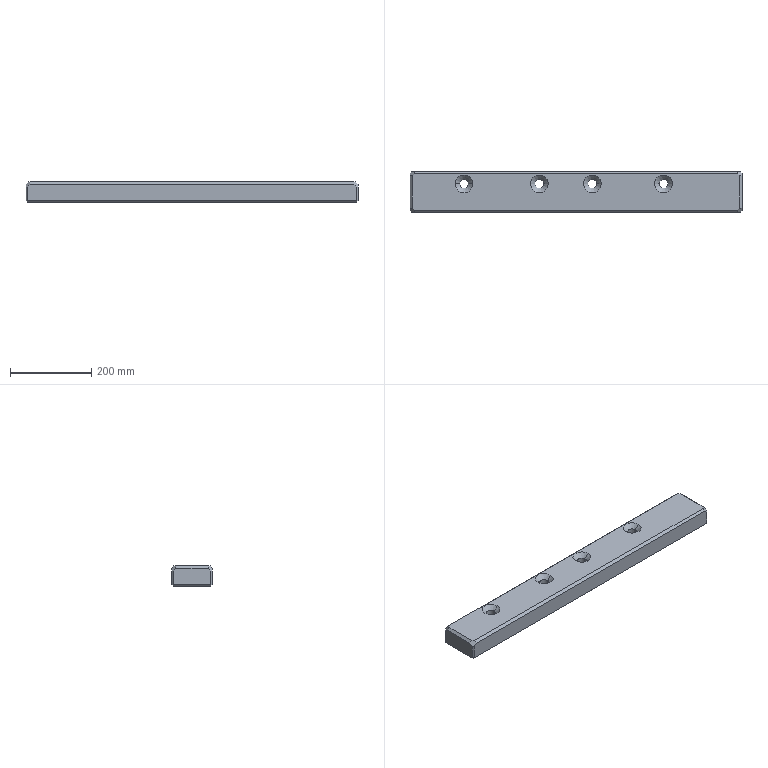Part | Creo | 1 solid | 50 faces | box 815 x 100 x 49.3 mm | volume 3878023 mm3 | plane 26 | cone 16 | cylinder 8 | commonest cylinder face diameters 22 x8
STEP:
#1=CARTESIAN_POINT('',(0.,0.,0.));
#2=DIRECTION('',(0.,0.,1.));
#3=DIRECTION('',(1.,0.,0.));
#4=AXIS2_PLACEMENT_3D('',#1,#2,#3);
#5=CARTESIAN_POINT('',(-330.17,-424.056,305.059));
#6=VERTEX_POINT('',#5);
#7=CARTESIAN_POINT('',(-325.328,-428.899,305.059));
#8=VERTEX_POINT('',#7);
#9=CARTESIAN_POINT('',(-330.17,-424.056,305.059));
#10=DIRECTION('',(0.7071,-0.7071,0.));
#11=VECTOR('',#10,6.848);
#12=LINE('',#9,#11);
#13=EDGE_CURVE('',#6,#8,#12,.T.);
#14=ORIENTED_EDGE('',*,*,#13,.F.);
#15=CARTESIAN_POINT('',(-330.17,-345.199,305.059));
#16=VERTEX_POINT('',#15);
#17=CARTESIAN_POINT('',(-330.17,-424.056,305.059));
#18=DIRECTION('',(0.,1.,0.));
#19=VECTOR('',#18,78.858);
#20=LINE('',#17,#19);
#21=EDGE_CURVE('',#6,#16,#20,.T.);
#22=ORIENTED_EDGE('',*,*,#21,.T.);
#23=CARTESIAN_POINT('',(-325.328,-340.356,305.059));
#24=VERTEX_POINT('',#23);
#25=CARTESIAN_POINT('',(-330.17,-345.199,305.059));
#26=DIRECTION('',(0.7071,0.7071,0.));
#27=VECTOR('',#26,6.848);
#28=LINE('',#25,#27);
#29=EDGE_CURVE('',#16,#24,#28,.T.);
#30=ORIENTED_EDGE('',*,*,#29,.T.);
#31=CARTESIAN_POINT('',(468.53,-340.356,305.059));
#32=VERTEX_POINT('',#31);
#33=CARTESIAN_POINT('',(-325.328,-340.356,305.059));
#34=DIRECTION('',(1.,0.,0.));
#35=VECTOR('',#34,793.858);
#36=LINE('',#33,#35);
#37=EDGE_CURVE('',#24,#32,#36,.T.);
#38=ORIENTED_EDGE('',*,*,#37,.T.);
#39=CARTESIAN_POINT('',(473.372,-345.199,305.059));
#40=VERTEX_POINT('',#39);
#41=CARTESIAN_POINT('',(473.372,-345.199,305.059));
#42=DIRECTION('',(-0.7071,0.7071,0.));
#43=VECTOR('',#42,6.848);
#44=LINE('',#41,#43);
#45=EDGE_CURVE('',#40,#32,#44,.T.);
#46=ORIENTED_EDGE('',*,*,#45,.F.);
#47=CARTESIAN_POINT('',(473.372,-424.056,305.059));
#48=VERTEX_POINT('',#47);
#49=CARTESIAN_POINT('',(473.372,-345.199,305.059));
#50=DIRECTION('',(0.,-1.,0.));
#51=VECTOR('',#50,78.858);
#52=LINE('',#49,#51);
#53=EDGE_CURVE('',#40,#48,#52,.T.);
#54=ORIENTED_EDGE('',*,*,#53,.T.);
#55=CARTESIAN_POINT('',(468.53,-428.899,305.059));
#56=VERTEX_POINT('',#55);
#57=CARTESIAN_POINT('',(468.53,-428.899,305.059));
#58=DIRECTION('',(0.7071,0.7071,0.));
#59=VECTOR('',#58,6.848);
#60=LINE('',#57,#59);
#61=EDGE_CURVE('',#56,#48,#60,.T.);
#62=ORIENTED_EDGE('',*,*,#61,.F.);
#63=CARTESIAN_POINT('',(468.53,-428.899,305.059));
#64=DIRECTION('',(-1.,0.,0.));
#65=VECTOR('',#64,793.858);
#66=LINE('',#63,#65);
#67=EDGE_CURVE('',#56,#8,#66,.T.);
#68=ORIENTED_EDGE('',*,*,#67,.T.);
#69=EDGE_LOOP('',(#14,#22,#30,#38,#46,#54,#62,#68));
#70=FACE_OUTER_BOUND('',#69,.F.);
#71=CARTESIAN_POINT('',(-181.599,-364.627,305.059));
#72=VERTEX_POINT('',#71);
#73=CARTESIAN_POINT('',(-225.199,-364.627,305.059));
#74=VERTEX_POINT('',#73);
#75=CARTESIAN_POINT('',(-203.399,-364.627,305.059));
#76=DIRECTION('',(0.,0.,-1.));
#77=DIRECTION('',(1.,0.,0.));
#78=AXIS2_PLACEMENT_3D('',#75,#76,#77);
#79=CIRCLE('',#78,21.8);
#80=EDGE_CURVE('',#72,#74,#79,.T.);
#81=ORIENTED_EDGE('',*,*,#80,.F.);
#82=CARTESIAN_POINT('',(-203.399,-364.627,305.059));
#83=DIRECTION('',(0.,0.,-1.));
#84=DIRECTION('',(-1.,0.,0.));
#85=AXIS2_PLACEMENT_3D('',#82,#83,#84);
#86=CIRCLE('',#85,21.8);
#87=EDGE_CURVE('',#74,#72,#86,.T.);
#88=ORIENTED_EDGE('',*,*,#87,.F.);
#89=EDGE_LOOP('',(#81,#88));
#90=FACE_BOUND('',#89,.F.);
#91=CARTESIAN_POINT('',(3.401,-364.627,305.059));
#92=VERTEX_POINT('',#91);
#93=CARTESIAN_POINT('',(-40.199,-364.627,305.059));
#94=VERTEX_POINT('',#93);
#95=CARTESIAN_POINT('',(-18.399,-364.627,305.059));
#96=DIRECTION('',(0.,0.,-1.));
#97=DIRECTION('',(1.,0.,0.));
#98=AXIS2_PLACEMENT_3D('',#95,#96,#97);
#99=CIRCLE('',#98,21.8);
#100=EDGE_CURVE('',#92,#94,#99,.T.);
#101=ORIENTED_EDGE('',*,*,#100,.F.);
#102=CARTESIAN_POINT('',(-18.399,-364.627,305.059));
#103=DIRECTION('',(0.,0.,-1.));
#104=DIRECTION('',(-1.,0.,0.));
#105=AXIS2_PLACEMENT_3D('',#102,#103,#104);
#106=CIRCLE('',#105,21.8);
#107=EDGE_CURVE('',#94,#92,#106,.T.);
#108=ORIENTED_EDGE('',*,*,#107,.F.);
#109=EDGE_LOOP('',(#101,#108));
#110=FACE_BOUND('',#109,.F.);
#111=CARTESIAN_POINT('',(133.401,-364.627,305.059));
#112=VERTEX_POINT('',#111);
#113=CARTESIAN_POINT('',(89.801,-364.627,305.059));
#114=VERTEX_POINT('',#113);
#115=CARTESIAN_POINT('',(111.601,-364.627,305.059));
#116=DIRECTION('',(0.,0.,-1.));
#117=DIRECTION('',(1.,0.,0.));
#118=AXIS2_PLACEMENT_3D('',#115,#116,#117);
#119=CIRCLE('',#118,21.8);
#120=EDGE_CURVE('',#112,#114,#119,.T.);
#121=ORIENTED_EDGE('',*,*,#120,.F.);
#122=CARTESIAN_POINT('',(111.601,-364.627,305.059));
#123=DIRECTION('',(0.,0.,-1.));
#124=DIRECTION('',(-1.,0.,0.));
#125=AXIS2_PLACEMENT_3D('',#122,#123,#124);
#126=CIRCLE('',#125,21.8);
#127=EDGE_CURVE('',#114,#112,#126,.T.);
#128=ORIENTED_EDGE('',*,*,#127,.F.);
#129=EDGE_LOOP('',(#121,#128));
#130=FACE_BOUND('',#129,.F.);
#131=CARTESIAN_POINT('',(308.401,-364.627,305.059));
#132=VERTEX_POINT('',#131);
#133=CARTESIAN_POINT('',(264.801,-364.627,305.059));
#134=VERTEX_POINT('',#133);
#135=CARTESIAN_POINT('',(286.601,-364.627,305.059));
#136=DIRECTION('',(0.,0.,-1.));
#137=DIRECTION('',(1.,0.,0.));
#138=AXIS2_PLACEMENT_3D('',#135,#136,#137);
#139=CIRCLE('',#138,21.8);
#140=EDGE_CURVE('',#132,#134,#139,.T.);
#141=ORIENTED_EDGE('',*,*,#140,.F.);
#142=CARTESIAN_POINT('',(286.601,-364.627,305.059));
#143=DIRECTION('',(0.,0.,-1.));
#144=DIRECTION('',(-1.,0.,0.));
#145=AXIS2_PLACEMENT_3D('',#142,#143,#144);
#146=CIRCLE('',#145,21.8);
#147=EDGE_CURVE('',#134,#132,#146,.T.);
#148=ORIENTED_EDGE('',*,*,#147,.F.);
#149=EDGE_LOOP('',(#141,#148));
#150=FACE_BOUND('',#149,.F.);
#151=CARTESIAN_POINT('',(479.101,-434.627,305.059));
#152=DIRECTION('',(0.,0.,1.));
#153=DIRECTION('',(1.,0.,0.));
#154=AXIS2_PLACEMENT_3D('',#151,#152,#153);
#155=PLANE('',#154);
#156=ADVANCED_FACE('',(#70,#90,#110,#130,#150),#155,.T.);
#157=CARTESIAN_POINT('',(-325.328,-434.627,299.33));
#158=VERTEX_POINT('',#157);
#159=CARTESIAN_POINT('',(-325.328,-434.627,299.33));
#160=DIRECTION('',(0.,0.7071,0.7071));
#161=VECTOR('',#160,8.102);
#162=LINE('',#159,#161);
#163=EDGE_CURVE('',#158,#8,#162,.T.);
#164=ORIENTED_EDGE('',*,*,#163,.F.);
#165=CARTESIAN_POINT('',(-332.399,-434.627,292.259));
#166=VERTEX_POINT('',#165);
#167=CARTESIAN_POINT('',(-325.328,-434.627,299.33));
#168=DIRECTION('',(-0.7071,0.,-0.7071));
#169=VECTOR('',#168,10.);
#170=LINE('',#167,#169);
#171=EDGE_CURVE('',#158,#166,#170,.T.);
#172=ORIENTED_EDGE('',*,*,#171,.T.);
#173=CARTESIAN_POINT('',(-335.899,-431.127,292.259));
#174=VERTEX_POINT('',#173);
#175=CARTESIAN_POINT('',(-335.899,-431.127,292.259));
#176=DIRECTION('',(0.7071,-0.7071,0.));
#177=VECTOR('',#176,4.95);
#178=LINE('',#175,#177);
#179=EDGE_CURVE('',#174,#166,#178,.T.);
#180=ORIENTED_EDGE('',*,*,#179,.F.);
#181=CARTESIAN_POINT('',(-335.899,-424.056,299.33));
#182=VERTEX_POINT('',#181);
#183=CARTESIAN_POINT('',(-335.899,-431.127,292.259));
#184=DIRECTION('',(0.,0.7071,0.7071));
#185=VECTOR('',#184,10.);
#186=LINE('',#183,#185);
#187=EDGE_CURVE('',#174,#182,#186,.T.);
#188=ORIENTED_EDGE('',*,*,#187,.T.);
#189=CARTESIAN_POINT('',(-330.17,-424.056,305.059));
#190=DIRECTION('',(-0.7071,0.,-0.7071));
#191=VECTOR('',#190,8.102);
#192=LINE('',#189,#191);
#193=EDGE_CURVE('',#6,#182,#192,.T.);
#194=ORIENTED_EDGE('',*,*,#193,.F.);
#195=ORIENTED_EDGE('',*,*,#13,.T.);
#196=EDGE_LOOP('',(#164,#172,#180,#188,#194,#195));
#197=FACE_OUTER_BOUND('',#196,.F.);
#198=CARTESIAN_POINT('',(-335.899,-431.127,292.259));
#199=DIRECTION('',(-0.5774,-0.5774,0.5774));
#200=DIRECTION('',(0.,-0.7071,-0.7071));
#201=AXIS2_PLACEMENT_3D('',#198,#199,#200);
#202=PLANE('',#201);
#203=ADVANCED_FACE('',(#197),#202,.T.);
#204=ORIENTED_EDGE('',*,*,#67,.F.);
#205=CARTESIAN_POINT('',(468.53,-434.627,299.33));
#206=VERTEX_POINT('',#205);
#207=CARTESIAN_POINT('',(468.53,-428.899,305.059));
#208=DIRECTION('',(0.,-0.7071,-0.7071));
#209=VECTOR('',#208,8.102);
#210=LINE('',#207,#209);
#211=EDGE_CURVE('',#56,#206,#210,.T.);
#212=ORIENTED_EDGE('',*,*,#211,.T.);
#213=CARTESIAN_POINT('',(-325.328,-434.627,299.33));
#214=DIRECTION('',(1.,0.,0.));
#215=VECTOR('',#214,793.858);
#216=LINE('',#213,#215);
#217=EDGE_CURVE('',#158,#206,#216,.T.);
#218=ORIENTED_EDGE('',*,*,#217,.F.);
#219=ORIENTED_EDGE('',*,*,#163,.T.);
#220=EDGE_LOOP('',(#204,#212,#218,#219));
#221=FACE_OUTER_BOUND('',#220,.F.);
#222=CARTESIAN_POINT('',(479.101,-438.163,295.794));
#223=DIRECTION('',(0.,0.7071,-0.7071));
#224=DIRECTION('',(0.,0.7071,0.7071));
#225=AXIS2_PLACEMENT_3D('',#222,#223,#224);
#226=PLANE('',#225);
#227=ADVANCED_FACE('',(#221),#226,.F.);
#228=CARTESIAN_POINT('',(479.101,-424.056,299.33));
#229=VERTEX_POINT('',#228);
#230=CARTESIAN_POINT('',(479.101,-424.056,299.33));
#231=DIRECTION('',(-0.7071,0.,0.7071));
#232=VECTOR('',#231,8.102);
#233=LINE('',#230,#232);
#234=EDGE_CURVE('',#229,#48,#233,.T.);
#235=ORIENTED_EDGE('',*,*,#234,.F.);
#236=CARTESIAN_POINT('',(479.101,-431.127,292.259));
#237=VERTEX_POINT('',#236);
#238=CARTESIAN_POINT('',(479.101,-424.056,299.33));
#239=DIRECTION('',(0.,-0.7071,-0.7071));
#240=VECTOR('',#239,10.);
#241=LINE('',#238,#240);
#242=EDGE_CURVE('',#229,#237,#241,.T.);
#243=ORIENTED_EDGE('',*,*,#242,.T.);
#244=CARTESIAN_POINT('',(475.601,-434.627,292.259));
#245=VERTEX_POINT('',#244);
#246=CARTESIAN_POINT('',(475.601,-434.627,292.259));
#247=DIRECTION('',(0.7071,0.7071,0.));
#248=VECTOR('',#247,4.95);
#249=LINE('',#246,#248);
#250=EDGE_CURVE('',#245,#237,#249,.T.);
#251=ORIENTED_EDGE('',*,*,#250,.F.);
#252=CARTESIAN_POINT('',(475.601,-434.627,292.259));
#253=DIRECTION('',(-0.7071,0.,0.7071));
#254=VECTOR('',#253,10.);
#255=LINE('',#252,#254);
#256=EDGE_CURVE('',#245,#206,#255,.T.);
#257=ORIENTED_EDGE('',*,*,#256,.T.);
#258=ORIENTED_EDGE('',*,*,#211,.F.);
#259=ORIENTED_EDGE('',*,*,#61,.T.);
#260=EDGE_LOOP('',(#235,#243,#251,#257,#258,#259));
#261=FACE_OUTER_BOUND('',#260,.F.);
#262=CARTESIAN_POINT('',(479.101,-431.127,292.259));
#263=DIRECTION('',(0.5774,-0.5774,0.5774));
#264=DIRECTION('',(0.7071,0.,-0.7071));
#265=AXIS2_PLACEMENT_3D('',#262,#263,#264);
#266=PLANE('',#265);
#267=ADVANCED_FACE('',(#261),#266,.T.);
#268=ORIENTED_EDGE('',*,*,#53,.F.);
#269=CARTESIAN_POINT('',(479.101,-345.199,299.33));
#270=VERTEX_POINT('',#269);
#271=CARTESIAN_POINT('',(473.372,-345.199,305.059));
#272=DIRECTION('',(0.7071,0.,-0.7071));
#273=VECTOR('',#272,8.102);
#274=LINE('',#271,#273);
#275=EDGE_CURVE('',#40,#270,#274,.T.);
#276=ORIENTED_EDGE('',*,*,#275,.T.);
#277=CARTESIAN_POINT('',(479.101,-424.056,299.33));
#278=DIRECTION('',(0.,1.,0.));
#279=VECTOR('',#278,78.858);
#280=LINE('',#277,#279);
#281=EDGE_CURVE('',#229,#270,#280,.T.);
#282=ORIENTED_EDGE('',*,*,#281,.F.);
#283=ORIENTED_EDGE('',*,*,#234,.T.);
#284=EDGE_LOOP('',(#268,#276,#282,#283));
#285=FACE_OUTER_BOUND('',#284,.F.);
#286=CARTESIAN_POINT('',(479.136,-434.627,299.294));
#287=DIRECTION('',(0.7071,0.,0.7071));
#288=DIRECTION('',(0.7071,0.,-0.7071));
#289=AXIS2_PLACEMENT_3D('',#286,#287,#288);
#290=PLANE('',#289);
#291=ADVANCED_FACE('',(#285),#290,.T.);
#292=CARTESIAN_POINT('',(468.53,-334.627,299.33));
#293=VERTEX_POINT('',#292);
#294=CARTESIAN_POINT('',(468.53,-334.627,299.33));
#295=DIRECTION('',(0.,-0.7071,0.7071));
#296=VECTOR('',#295,8.102);
#297=LINE('',#294,#296);
#298=EDGE_CURVE('',#293,#32,#297,.T.);
#299=ORIENTED_EDGE('',*,*,#298,.F.);
#300=CARTESIAN_POINT('',(475.601,-334.627,292.259));
#301=VERTEX_POINT('',#300);
#302=CARTESIAN_POINT('',(468.53,-334.627,299.33));
#303=DIRECTION('',(0.7071,0.,-0.7071));
#304=VECTOR('',#303,10.);
#305=LINE('',#302,#304);
#306=EDGE_CURVE('',#293,#301,#305,.T.);
#307=ORIENTED_EDGE('',*,*,#306,.T.);
#308=CARTESIAN_POINT('',(479.101,-338.127,292.259));
#309=VERTEX_POINT('',#308);
#310=CARTESIAN_POINT('',(479.101,-338.127,292.259));
#311=DIRECTION('',(-0.7071,0.7071,0.));
#312=VECTOR('',#311,4.95);
#313=LINE('',#310,#312);
#314=EDGE_CURVE('',#309,#301,#313,.T.);
#315=ORIENTED_EDGE('',*,*,#314,.F.);
#316=CARTESIAN_POINT('',(479.101,-345.199,299.33));
#317=DIRECTION('',(0.,0.7071,-0.7071));
#318=VECTOR('',#317,10.);
#319=LINE('',#316,#318);
#320=EDGE_CURVE('',#270,#309,#319,.T.);
#321=ORIENTED_EDGE('',*,*,#320,.F.);
#322=ORIENTED_EDGE('',*,*,#275,.F.);
#323=ORIENTED_EDGE('',*,*,#45,.T.);
#324=EDGE_LOOP('',(#299,#307,#315,#321,#322,#323));
#325=FACE_OUTER_BOUND('',#324,.F.);
#326=CARTESIAN_POINT('',(475.601,-338.127,295.759));
#327=DIRECTION('',(0.5774,0.5774,0.5774));
#328=DIRECTION('',(0.7071,0.,-0.7071));
#329=AXIS2_PLACEMENT_3D('',#326,#327,#328);
#330=PLANE('',#329);
#331=ADVANCED_FACE('',(#325),#330,.T.);
#332=CARTESIAN_POINT('',(-325.328,-334.627,299.33));
#333=VERTEX_POINT('',#332);
#334=CARTESIAN_POINT('',(-325.328,-340.356,305.059));
#335=DIRECTION('',(0.,0.7071,-0.7071));
#336=VECTOR('',#335,8.102);
#337=LINE('',#334,#336);
#338=EDGE_CURVE('',#24,#333,#337,.T.);
#339=ORIENTED_EDGE('',*,*,#338,.T.);
#340=CARTESIAN_POINT('',(468.53,-334.627,299.33));
#341=DIRECTION('',(-1.,0.,0.));
#342=VECTOR('',#341,793.858);
#343=LINE('',#340,#342);
#344=EDGE_CURVE('',#293,#333,#343,.T.);
#345=ORIENTED_EDGE('',*,*,#344,.F.);
#346=ORIENTED_EDGE('',*,*,#298,.T.);
#347=ORIENTED_EDGE('',*,*,#37,.F.);
#348=EDGE_LOOP('',(#339,#345,#346,#347));
#349=FACE_OUTER_BOUND('',#348,.F.);
#350=CARTESIAN_POINT('',(479.101,-334.592,299.294));
#351=DIRECTION('',(0.,0.7071,0.7071));
#352=DIRECTION('',(0.,-0.7071,0.7071));
#353=AXIS2_PLACEMENT_3D('',#350,#351,#352);
#354=PLANE('',#353);
#355=ADVANCED_FACE('',(#349),#354,.T.);
#356=ORIENTED_EDGE('',*,*,#29,.F.);
#357=CARTESIAN_POINT('',(-335.899,-345.199,299.33));
#358=VERTEX_POINT('',#357);
#359=CARTESIAN_POINT('',(-335.899,-345.199,299.33));
#360=DIRECTION('',(0.7071,0.,0.7071));
#361=VECTOR('',#360,8.102);
#362=LINE('',#359,#361);
#363=EDGE_CURVE('',#358,#16,#362,.T.);
#364=ORIENTED_EDGE('',*,*,#363,.F.);
#365=CARTESIAN_POINT('',(-335.899,-338.127,292.259));
#366=VERTEX_POINT('',#365);
#367=CARTESIAN_POINT('',(-335.899,-345.199,299.33));
#368=DIRECTION('',(0.,0.7071,-0.7071));
#369=VECTOR('',#368,10.);
#370=LINE('',#367,#369);
#371=EDGE_CURVE('',#358,#366,#370,.T.);
#372=ORIENTED_EDGE('',*,*,#371,.T.);
#373=CARTESIAN_POINT('',(-332.399,-334.627,292.259));
#374=VERTEX_POINT('',#373);
#375=CARTESIAN_POINT('',(-332.399,-334.627,292.259));
#376=DIRECTION('',(-0.7071,-0.7071,0.));
#377=VECTOR('',#376,4.95);
#378=LINE('',#375,#377);
#379=EDGE_CURVE('',#374,#366,#378,.T.);
#380=ORIENTED_EDGE('',*,*,#379,.F.);
#381=CARTESIAN_POINT('',(-325.328,-334.627,299.33));
#382=DIRECTION('',(-0.7071,0.,-0.7071));
#383=VECTOR('',#382,10.);
#384=LINE('',#381,#383);
#385=EDGE_CURVE('',#333,#374,#384,.T.);
#386=ORIENTED_EDGE('',*,*,#385,.F.);
#387=ORIENTED_EDGE('',*,*,#338,.F.);
#388=EDGE_LOOP('',(#356,#364,#372,#380,#386,#387));
#389=FACE_OUTER_BOUND('',#388,.F.);
#390=CARTESIAN_POINT('',(-332.399,-338.127,295.759));
#391=DIRECTION('',(-0.5774,0.5774,0.5774));
#392=DIRECTION('',(0.,-0.7071,0.7071));
#393=AXIS2_PLACEMENT_3D('',#390,#391,#392);
#394=PLANE('',#393);
#395=ADVANCED_FACE('',(#389),#394,.T.);
#396=ORIENTED_EDGE('',*,*,#21,.F.);
#397=ORIENTED_EDGE('',*,*,#193,.T.);
#398=CARTESIAN_POINT('',(-335.899,-345.199,299.33));
#399=DIRECTION('',(0.,-1.,0.));
#400=VECTOR('',#399,78.858);
#401=LINE('',#398,#400);
#402=EDGE_CURVE('',#358,#182,#401,.T.);
#403=ORIENTED_EDGE('',*,*,#402,.F.);
#404=ORIENTED_EDGE('',*,*,#363,.T.);
#405=EDGE_LOOP('',(#396,#397,#403,#404));
#406=FACE_OUTER_BOUND('',#405,.F.);
#407=CARTESIAN_POINT('',(-339.435,-434.627,295.794));
#408=DIRECTION('',(0.7071,0.,-0.7071));
#409=DIRECTION('',(-0.7071,0.,-0.7071));
#410=AXIS2_PLACEMENT_3D('',#407,#408,#409);
#411=PLANE('',#410);
#412=ADVANCED_FACE('',(#406),#411,.F.);
#413=CARTESIAN_POINT('',(-335.899,-338.127,259.259));
#414=VERTEX_POINT('',#413);
#415=CARTESIAN_POINT('',(-335.899,-338.127,259.259));
#416=DIRECTION('',(0.,0.,1.));
#417=VECTOR('',#416,33.);
#418=LINE('',#415,#417);
#419=EDGE_CURVE('',#414,#366,#418,.T.);
#420=ORIENTED_EDGE('',*,*,#419,.T.);
#421=ORIENTED_EDGE('',*,*,#371,.F.);
#422=ORIENTED_EDGE('',*,*,#402,.T.);
#423=ORIENTED_EDGE('',*,*,#187,.F.);
#424=CARTESIAN_POINT('',(-335.899,-431.127,259.259));
#425=VERTEX_POINT('',#424);
#426=CARTESIAN_POINT('',(-335.899,-431.127,292.259));
#427=DIRECTION('',(0.,0.,-1.));
#428=VECTOR('',#427,33.);
#429=LINE('',#426,#428);
#430=EDGE_CURVE('',#174,#425,#429,.T.);
#431=ORIENTED_EDGE('',*,*,#430,.T.);
#432=CARTESIAN_POINT('',(-335.899,-431.127,259.259));
#433=DIRECTION('',(0.,1.,0.));
#434=VECTOR('',#433,93.);
#435=LINE('',#432,#434);
#436=EDGE_CURVE('',#425,#414,#435,.T.);
#437=ORIENTED_EDGE('',*,*,#436,.T.);
#438=EDGE_LOOP('',(#420,#421,#422,#423,#431,#437));
#439=FACE_OUTER_BOUND('',#438,.F.);
#440=CARTESIAN_POINT('',(-335.899,-434.627,295.759));
#441=DIRECTION('',(-1.,0.,0.));
#442=DIRECTION('',(0.,0.,1.));
#443=AXIS2_PLACEMENT_3D('',#440,#441,#442);
#444=PLANE('',#443);
#445=ADVANCED_FACE('',(#439),#444,.T.);
#446=CARTESIAN_POINT('',(-332.399,-334.627,259.259));
#447=VERTEX_POINT('',#446);
#448=CARTESIAN_POINT('',(-335.899,-338.127,259.259));
#449=DIRECTION('',(0.7071,0.7071,0.));
#450=VECTOR('',#449,4.95);
#451=LINE('',#448,#450);
#452=EDGE_CURVE('',#414,#447,#451,.T.);
#453=ORIENTED_EDGE('',*,*,#452,.T.);
#454=CARTESIAN_POINT('',(-332.399,-334.627,292.259));
#455=DIRECTION('',(0.,0.,-1.));
#456=VECTOR('',#455,33.);
#457=LINE('',#454,#456);
#458=EDGE_CURVE('',#374,#447,#457,.T.);
#459=ORIENTED_EDGE('',*,*,#458,.F.);
#460=ORIENTED_EDGE('',*,*,#379,.T.);
#461=ORIENTED_EDGE('',*,*,#419,.F.);
#462=EDGE_LOOP('',(#453,#459,#460,#461));
#463=FACE_OUTER_BOUND('',#462,.F.);
#464=CARTESIAN_POINT('',(-335.899,-338.127,295.759));
#465=DIRECTION('',(-0.7071,0.7071,0.));
#466=DIRECTION('',(-0.7071,-0.7071,0.));
#467=AXIS2_PLACEMENT_3D('',#464,#465,#466);
#468=PLANE('',#467);
#469=ADVANCED_FACE('',(#463),#468,.T.);
#470=CARTESIAN_POINT('',(-332.399,-338.127,255.759));
#471=VERTEX_POINT('',#470);
#472=CARTESIAN_POINT('',(-332.399,-334.627,259.259));
#473=DIRECTION('',(0.,-0.7071,-0.7071));
#474=VECTOR('',#473,4.95);
#475=LINE('',#472,#474);
#476=EDGE_CURVE('',#447,#471,#475,.T.);
#477=ORIENTED_EDGE('',*,*,#476,.F.);
#478=ORIENTED_EDGE('',*,*,#452,.F.);
#479=CARTESIAN_POINT('',(-332.399,-338.127,255.759));
#480=DIRECTION('',(-0.7071,0.,0.7071));
#481=VECTOR('',#480,4.95);
#482=LINE('',#479,#481);
#483=EDGE_CURVE('',#471,#414,#482,.T.);
#484=ORIENTED_EDGE('',*,*,#483,.F.);
#485=EDGE_LOOP('',(#477,#478,#484));
#486=FACE_OUTER_BOUND('',#485,.F.);
#487=CARTESIAN_POINT('',(-332.399,-338.127,255.759));
#488=DIRECTION('',(-0.5774,0.5774,-0.5774));
#489=DIRECTION('',(0.,0.7071,0.7071));
#490=AXIS2_PLACEMENT_3D('',#487,#488,#489);
#491=PLANE('',#490);
#492=ADVANCED_FACE('',(#486),#491,.T.);
#493=ORIENTED_EDGE('',*,*,#476,.T.);
#494=CARTESIAN_POINT('',(475.601,-338.127,255.759));
#495=VERTEX_POINT('',#494);
#496=CARTESIAN_POINT('',(475.601,-338.127,255.759));
#497=DIRECTION('',(-1.,0.,0.));
#498=VECTOR('',#497,808.);
#499=LINE('',#496,#498);
#500=EDGE_CURVE('',#495,#471,#499,.T.);
#501=ORIENTED_EDGE('',*,*,#500,.F.);
#502=CARTESIAN_POINT('',(475.601,-334.627,259.259));
#503=VERTEX_POINT('',#502);
#504=CARTESIAN_POINT('',(475.601,-338.127,255.759));
#505=DIRECTION('',(0.,0.7071,0.7071));
#506=VECTOR('',#505,4.95);
#507=LINE('',#504,#506);
#508=EDGE_CURVE('',#495,#503,#507,.T.);
#509=ORIENTED_EDGE('',*,*,#508,.T.);
#510=CARTESIAN_POINT('',(-332.399,-334.627,259.259));
#511=DIRECTION('',(1.,0.,0.));
#512=VECTOR('',#511,808.);
#513=LINE('',#510,#512);
#514=EDGE_CURVE('',#447,#503,#513,.T.);
#515=ORIENTED_EDGE('',*,*,#514,.F.);
#516=EDGE_LOOP('',(#493,#501,#509,#515));
#517=FACE_OUTER_BOUND('',#516,.F.);
#518=CARTESIAN_POINT('',(479.101,-334.627,259.259));
#519=DIRECTION('',(0.,-0.7071,0.7071));
#520=DIRECTION('',(0.,-0.7071,-0.7071));
#521=AXIS2_PLACEMENT_3D('',#518,#519,#520);
#522=PLANE('',#521);
#523=ADVANCED_FACE('',(#517),#522,.F.);
#524=CARTESIAN_POINT('',(-332.399,-431.127,255.759));
#525=VERTEX_POINT('',#524);
#526=CARTESIAN_POINT('',(475.601,-431.127,255.759));
#527=VERTEX_POINT('',#526);
#528=CARTESIAN_POINT('',(-332.399,-431.127,255.759));
#529=DIRECTION('',(1.,0.,0.));
#530=VECTOR('',#529,808.);
#531=LINE('',#528,#530);
#532=EDGE_CURVE('',#525,#527,#531,.T.);
#533=ORIENTED_EDGE('',*,*,#532,.T.);
#534=CARTESIAN_POINT('',(475.601,-431.127,255.759));
#535=DIRECTION('',(0.,1.,0.));
#536=VECTOR('',#535,93.);
#537=LINE('',#534,#536);
#538=EDGE_CURVE('',#527,#495,#537,.T.);
#539=ORIENTED_EDGE('',*,*,#538,.T.);
#540=ORIENTED_EDGE('',*,*,#500,.T.);
#541=CARTESIAN_POINT('',(-332.399,-338.127,255.759));
#542=DIRECTION('',(0.,-1.,0.));
#543=VECTOR('',#542,93.);
#544=LINE('',#541,#543);
#545=EDGE_CURVE('',#471,#525,#544,.T.);
#546=ORIENTED_EDGE('',*,*,#545,.T.);
#547=EDGE_LOOP('',(#533,#539,#540,#546));
#548=FACE_OUTER_BOUND('',#547,.F.);
#549=CARTESIAN_POINT('',(124.101,-364.627,255.759));
#550=VERTEX_POINT('',#549);
#551=CARTESIAN_POINT('',(99.101,-364.627,255.759));
#552=VERTEX_POINT('',#551);
#553=CARTESIAN_POINT('',(111.601,-364.627,255.759));
#554=DIRECTION('',(0.,0.,1.));
#555=DIRECTION('',(1.,0.,0.));
#556=AXIS2_PLACEMENT_3D('',#553,#554,#555);
#557=CIRCLE('',#556,12.5);
#558=EDGE_CURVE('',#550,#552,#557,.T.);
#559=ORIENTED_EDGE('',*,*,#558,.F.);
#560=CARTESIAN_POINT('',(111.601,-364.627,255.759));
#561=DIRECTION('',(0.,0.,1.));
#562=DIRECTION('',(-1.,0.,0.));
#563=AXIS2_PLACEMENT_3D('',#560,#561,#562);
#564=CIRCLE('',#563,12.5);
#565=EDGE_CURVE('',#552,#550,#564,.T.);
#566=ORIENTED_EDGE('',*,*,#565,.F.);
#567=EDGE_LOOP('',(#559,#566));
#568=FACE_BOUND('',#567,.F.);
#569=CARTESIAN_POINT('',(-5.899,-364.627,255.759));
#570=VERTEX_POINT('',#569);
#571=CARTESIAN_POINT('',(-30.899,-364.627,255.759));
#572=VERTEX_POINT('',#571);
#573=CARTESIAN_POINT('',(-18.399,-364.627,255.759));
#574=DIRECTION('',(0.,0.,1.));
#575=DIRECTION('',(1.,0.,0.));
#576=AXIS2_PLACEMENT_3D('',#573,#574,#575);
#577=CIRCLE('',#576,12.5);
#578=EDGE_CURVE('',#570,#572,#577,.T.);
#579=ORIENTED_EDGE('',*,*,#578,.F.);
#580=CARTESIAN_POINT('',(-18.399,-364.627,255.759));
#581=DIRECTION('',(0.,0.,1.));
#582=DIRECTION('',(-1.,0.,0.));
#583=AXIS2_PLACEMENT_3D('',#580,#581,#582);
#584=CIRCLE('',#583,12.5);
#585=EDGE_CURVE('',#572,#570,#584,.T.);
#586=ORIENTED_EDGE('',*,*,#585,.F.);
#587=EDGE_LOOP('',(#579,#586));
#588=FACE_BOUND('',#587,.F.);
#589=CARTESIAN_POINT('',(-190.899,-364.627,255.759));
#590=VERTEX_POINT('',#589);
#591=CARTESIAN_POINT('',(-215.899,-364.627,255.759));
#592=VERTEX_POINT('',#591);
#593=CARTESIAN_POINT('',(-203.399,-364.627,255.759));
#594=DIRECTION('',(0.,0.,1.));
#595=DIRECTION('',(1.,0.,0.));
#596=AXIS2_PLACEMENT_3D('',#593,#594,#595);
#597=CIRCLE('',#596,12.5);
#598=EDGE_CURVE('',#590,#592,#597,.T.);
#599=ORIENTED_EDGE('',*,*,#598,.F.);
#600=CARTESIAN_POINT('',(-203.399,-364.627,255.759));
#601=DIRECTION('',(0.,0.,1.));
#602=DIRECTION('',(-1.,0.,0.));
#603=AXIS2_PLACEMENT_3D('',#600,#601,#602);
#604=CIRCLE('',#603,12.5);
#605=EDGE_CURVE('',#592,#590,#604,.T.);
#606=ORIENTED_EDGE('',*,*,#605,.F.);
#607=EDGE_LOOP('',(#599,#606));
#608=FACE_BOUND('',#607,.F.);
#609=CARTESIAN_POINT('',(299.101,-364.627,255.759));
#610=VERTEX_POINT('',#609);
#611=CARTESIAN_POINT('',(274.101,-364.627,255.759));
#612=VERTEX_POINT('',#611);
#613=CARTESIAN_POINT('',(286.601,-364.627,255.759));
#614=DIRECTION('',(0.,0.,1.));
#615=DIRECTION('',(1.,0.,0.));
#616=AXIS2_PLACEMENT_3D('',#613,#614,#615);
#617=CIRCLE('',#616,12.5);
#618=EDGE_CURVE('',#610,#612,#617,.T.);
#619=ORIENTED_EDGE('',*,*,#618,.F.);
#620=CARTESIAN_POINT('',(286.601,-364.627,255.759));
#621=DIRECTION('',(0.,0.,1.));
#622=DIRECTION('',(-1.,0.,0.));
#623=AXIS2_PLACEMENT_3D('',#620,#621,#622);
#624=CIRCLE('',#623,12.5);
#625=EDGE_CURVE('',#612,#610,#624,.T.);
#626=ORIENTED_EDGE('',*,*,#625,.F.);
#627=EDGE_LOOP('',(#619,#626));
#628=FACE_BOUND('',#627,.F.);
#629=CARTESIAN_POINT('',(479.101,-434.627,255.759));
#630=DIRECTION('',(0.,0.,1.));
#631=DIRECTION('',(1.,0.,0.));
#632=AXIS2_PLACEMENT_3D('',#629,#630,#631);
#633=PLANE('',#632);
#634=ADVANCED_FACE('',(#548,#568,#588,#608,#628),#633,.F.);
#635=CARTESIAN_POINT('',(297.601,-364.627,257.259));
#636=VERTEX_POINT('',#635);
#637=CARTESIAN_POINT('',(275.601,-364.627,257.259));
#638=VERTEX_POINT('',#637);
#639=CARTESIAN_POINT('',(286.601,-364.627,257.259));
#640=DIRECTION('',(0.,0.,1.));
#641=DIRECTION('',(1.,0.,0.));
#642=AXIS2_PLACEMENT_3D('',#639,#640,#641);
#643=CIRCLE('',#642,11.);
#644=EDGE_CURVE('',#636,#638,#643,.T.);
#645=ORIENTED_EDGE('',*,*,#644,.F.);
#646=CARTESIAN_POINT('',(297.601,-364.627,257.259));
#647=DIRECTION('',(0.7071,0.,-0.7071));
#648=VECTOR('',#647,2.121);
#649=LINE('',#646,#648);
#650=EDGE_CURVE('',#636,#610,#649,.T.);
#651=ORIENTED_EDGE('',*,*,#650,.T.);
#652=ORIENTED_EDGE('',*,*,#618,.T.);
#653=CARTESIAN_POINT('',(275.601,-364.627,257.259));
#654=DIRECTION('',(-0.7071,0.,-0.7071));
#655=VECTOR('',#654,2.121);
#656=LINE('',#653,#655);
#657=EDGE_CURVE('',#638,#612,#656,.T.);
#658=ORIENTED_EDGE('',*,*,#657,.F.);
#659=EDGE_LOOP('',(#645,#651,#652,#658));
#660=FACE_OUTER_BOUND('',#659,.F.);
#661=CARTESIAN_POINT('',(286.601,-364.627,256.509));
#662=DIRECTION('',(0.,0.,-1.));
#663=DIRECTION('',(-1.,0.,0.));
#664=AXIS2_PLACEMENT_3D('',#661,#662,#663);
#665=CONICAL_SURFACE('',#664,11.75,45.);
#666=ADVANCED_FACE('',(#660),#665,.F.);
#667=CARTESIAN_POINT('',(275.601,-364.627,294.259));
#668=VERTEX_POINT('',#667);
#669=CARTESIAN_POINT('',(297.601,-364.627,294.259));
#670=VERTEX_POINT('',#669);
#671=CARTESIAN_POINT('',(286.601,-364.627,294.259));
#672=DIRECTION('',(0.,0.,-1.));
#673=DIRECTION('',(-1.,0.,0.));
#674=AXIS2_PLACEMENT_3D('',#671,#672,#673);
#675=CIRCLE('',#674,11.);
#676=EDGE_CURVE('',#668,#670,#675,.T.);
#677=ORIENTED_EDGE('',*,*,#676,.T.);
#678=CARTESIAN_POINT('',(297.601,-364.627,257.259));
#679=DIRECTION('',(0.,0.,1.));
#680=VECTOR('',#679,37.);
#681=LINE('',#678,#680);
#682=EDGE_CURVE('',#636,#670,#681,.T.);
#683=ORIENTED_EDGE('',*,*,#682,.F.);
#684=ORIENTED_EDGE('',*,*,#644,.T.);
#685=CARTESIAN_POINT('',(275.601,-364.627,257.259));
#686=DIRECTION('',(0.,0.,1.));
#687=VECTOR('',#686,37.);
#688=LINE('',#685,#687);
#689=EDGE_CURVE('',#638,#668,#688,.T.);
#690=ORIENTED_EDGE('',*,*,#689,.T.);
#691=EDGE_LOOP('',(#677,#683,#684,#690));
#692=FACE_OUTER_BOUND('',#691,.F.);
#693=CARTESIAN_POINT('',(286.601,-364.627,144.759));
#694=DIRECTION('',(0.,0.,1.));
#695=DIRECTION('',(1.,0.,0.));
#696=AXIS2_PLACEMENT_3D('',#693,#694,#695);
#697=CYLINDRICAL_SURFACE('',#696,11.);
#698=ADVANCED_FACE('',(#692),#697,.F.);
#699=ORIENTED_EDGE('',*,*,#676,.F.);
#700=CARTESIAN_POINT('',(275.601,-364.627,294.259));
#701=DIRECTION('',(-0.7071,0.,0.7071));
#702=VECTOR('',#701,15.274);
#703=LINE('',#700,#702);
#704=EDGE_CURVE('',#668,#134,#703,.T.);
#705=ORIENTED_EDGE('',*,*,#704,.T.);
#706=ORIENTED_EDGE('',*,*,#147,.T.);
#707=CARTESIAN_POINT('',(297.601,-364.627,294.259));
#708=DIRECTION('',(0.7071,0.,0.7071));
#709=VECTOR('',#708,15.274);
#710=LINE('',#707,#709);
#711=EDGE_CURVE('',#670,#132,#710,.T.);
#712=ORIENTED_EDGE('',*,*,#711,.F.);
#713=EDGE_LOOP('',(#699,#705,#706,#712));
#714=FACE_OUTER_BOUND('',#713,.F.);
#715=CARTESIAN_POINT('',(286.601,-364.627,299.659));
#716=DIRECTION('',(0.,0.,1.));
#717=DIRECTION('',(1.,0.,0.));
#718=AXIS2_PLACEMENT_3D('',#715,#716,#717);
#719=CONICAL_SURFACE('',#718,16.4,45.);
#720=ADVANCED_FACE('',(#714),#719,.F.);
#721=CARTESIAN_POINT('',(286.601,-364.627,294.259));
#722=DIRECTION('',(0.,0.,-1.));
#723=DIRECTION('',(1.,0.,0.));
#724=AXIS2_PLACEMENT_3D('',#721,#722,#723);
#725=CIRCLE('',#724,11.);
#726=EDGE_CURVE('',#670,#668,#725,.T.);
#727=ORIENTED_EDGE('',*,*,#726,.F.);
#728=ORIENTED_EDGE('',*,*,#711,.T.);
#729=ORIENTED_EDGE('',*,*,#140,.T.);
#730=ORIENTED_EDGE('',*,*,#704,.F.);
#731=EDGE_LOOP('',(#727,#728,#729,#730));
#732=FACE_OUTER_BOUND('',#731,.F.);
#733=CARTESIAN_POINT('',(286.601,-364.627,299.659));
#734=DIRECTION('',(0.,0.,1.));
#735=DIRECTION('',(1.,0.,0.));
#736=AXIS2_PLACEMENT_3D('',#733,#734,#735);
#737=CONICAL_SURFACE('',#736,16.4,45.);
#738=ADVANCED_FACE('',(#732),#737,.F.);
#739=ORIENTED_EDGE('',*,*,#726,.T.);
#740=ORIENTED_EDGE('',*,*,#689,.F.);
#741=CARTESIAN_POINT('',(286.601,-364.627,257.259));
#742=DIRECTION('',(0.,0.,1.));
#743=DIRECTION('',(-1.,0.,0.));
#744=AXIS2_PLACEMENT_3D('',#741,#742,#743);
#745=CIRCLE('',#744,11.);
#746=EDGE_CURVE('',#638,#636,#745,.T.);
#747=ORIENTED_EDGE('',*,*,#746,.T.);
#748=ORIENTED_EDGE('',*,*,#682,.T.);
#749=EDGE_LOOP('',(#739,#740,#747,#748));
#750=FACE_OUTER_BOUND('',#749,.F.);
#751=CARTESIAN_POINT('',(286.601,-364.627,144.759));
#752=DIRECTION('',(0.,0.,1.));
#753=DIRECTION('',(1.,0.,0.));
#754=AXIS2_PLACEMENT_3D('',#751,#752,#753);
#755=CYLINDRICAL_SURFACE('',#754,11.);
#756=ADVANCED_FACE('',(#750),#755,.F.);
#757=ORIENTED_EDGE('',*,*,#746,.F.);
#758=ORIENTED_EDGE('',*,*,#657,.T.);
#759=ORIENTED_EDGE('',*,*,#625,.T.);
#760=ORIENTED_EDGE('',*,*,#650,.F.);
#761=EDGE_LOOP('',(#757,#758,#759,#760));
#762=FACE_OUTER_BOUND('',#761,.F.);
#763=CARTESIAN_POINT('',(286.601,-364.627,256.509));
#764=DIRECTION('',(0.,0.,-1.));
#765=DIRECTION('',(-1.,0.,0.));
#766=AXIS2_PLACEMENT_3D('',#763,#764,#765);
#767=CONICAL_SURFACE('',#766,11.75,45.);
#768=ADVANCED_FACE('',(#762),#767,.F.);
#769=CARTESIAN_POINT('',(122.601,-364.627,257.259));
#770=VERTEX_POINT('',#769);
#771=CARTESIAN_POINT('',(100.601,-364.627,257.259));
#772=VERTEX_POINT('',#771);
#773=CARTESIAN_POINT('',(111.601,-364.627,257.259));
#774=DIRECTION('',(0.,0.,1.));
#775=DIRECTION('',(1.,0.,0.));
#776=AXIS2_PLACEMENT_3D('',#773,#774,#775);
#777=CIRCLE('',#776,11.);
#778=EDGE_CURVE('',#770,#772,#777,.T.);
#779=ORIENTED_EDGE('',*,*,#778,.F.);
#780=CARTESIAN_POINT('',(122.601,-364.627,257.259));
#781=DIRECTION('',(0.7071,0.,-0.7071));
#782=VECTOR('',#781,2.121);
#783=LINE('',#780,#782);
#784=EDGE_CURVE('',#770,#550,#783,.T.);
#785=ORIENTED_EDGE('',*,*,#784,.T.);
#786=ORIENTED_EDGE('',*,*,#558,.T.);
#787=CARTESIAN_POINT('',(100.601,-364.627,257.259));
#788=DIRECTION('',(-0.7071,0.,-0.7071));
#789=VECTOR('',#788,2.121);
#790=LINE('',#787,#789);
#791=EDGE_CURVE('',#772,#552,#790,.T.);
#792=ORIENTED_EDGE('',*,*,#791,.F.);
#793=EDGE_LOOP('',(#779,#785,#786,#792));
#794=FACE_OUTER_BOUND('',#793,.F.);
#795=CARTESIAN_POINT('',(111.601,-364.627,256.509));
#796=DIRECTION('',(0.,0.,-1.));
#797=DIRECTION('',(-1.,0.,0.));
#798=AXIS2_PLACEMENT_3D('',#795,#796,#797);
#799=CONICAL_SURFACE('',#798,11.75,45.);
#800=ADVANCED_FACE('',(#794),#799,.F.);
#801=CARTESIAN_POINT('',(100.601,-364.627,294.259));
#802=VERTEX_POINT('',#801);
#803=CARTESIAN_POINT('',(122.601,-364.627,294.259));
#804=VERTEX_POINT('',#803);
#805=CARTESIAN_POINT('',(111.601,-364.627,294.259));
#806=DIRECTION('',(0.,0.,-1.));
#807=DIRECTION('',(-1.,0.,0.));
#808=AXIS2_PLACEMENT_3D('',#805,#806,#807);
#809=CIRCLE('',#808,11.);
#810=EDGE_CURVE('',#802,#804,#809,.T.);
#811=ORIENTED_EDGE('',*,*,#810,.T.);
#812=CARTESIAN_POINT('',(122.601,-364.627,257.259));
#813=DIRECTION('',(0.,0.,1.));
#814=VECTOR('',#813,37.);
#815=LINE('',#812,#814);
#816=EDGE_CURVE('',#770,#804,#815,.T.);
#817=ORIENTED_EDGE('',*,*,#816,.F.);
#818=ORIENTED_EDGE('',*,*,#778,.T.);
#819=CARTESIAN_POINT('',(100.601,-364.627,257.259));
#820=DIRECTION('',(0.,0.,1.));
#821=VECTOR('',#820,37.);
#822=LINE('',#819,#821);
#823=EDGE_CURVE('',#772,#802,#822,.T.);
#824=ORIENTED_EDGE('',*,*,#823,.T.);
#825=EDGE_LOOP('',(#811,#817,#818,#824));
#826=FACE_OUTER_BOUND('',#825,.F.);
#827=CARTESIAN_POINT('',(111.601,-364.627,144.759));
#828=DIRECTION('',(0.,0.,1.));
#829=DIRECTION('',(1.,0.,0.));
#830=AXIS2_PLACEMENT_3D('',#827,#828,#829);
#831=CYLINDRICAL_SURFACE('',#830,11.);
#832=ADVANCED_FACE('',(#826),#831,.F.);
#833=ORIENTED_EDGE('',*,*,#810,.F.);
#834=CARTESIAN_POINT('',(100.601,-364.627,294.259));
#835=DIRECTION('',(-0.7071,0.,0.7071));
#836=VECTOR('',#835,15.274);
#837=LINE('',#834,#836);
#838=EDGE_CURVE('',#802,#114,#837,.T.);
#839=ORIENTED_EDGE('',*,*,#838,.T.);
#840=ORIENTED_EDGE('',*,*,#127,.T.);
#841=CARTESIAN_POINT('',(122.601,-364.627,294.259));
#842=DIRECTION('',(0.7071,0.,0.7071));
#843=VECTOR('',#842,15.274);
#844=LINE('',#841,#843);
#845=EDGE_CURVE('',#804,#112,#844,.T.);
#846=ORIENTED_EDGE('',*,*,#845,.F.);
#847=EDGE_LOOP('',(#833,#839,#840,#846));
#848=FACE_OUTER_BOUND('',#847,.F.);
#849=CARTESIAN_POINT('',(111.601,-364.627,299.659));
#850=DIRECTION('',(0.,0.,1.));
#851=DIRECTION('',(1.,0.,0.));
#852=AXIS2_PLACEMENT_3D('',#849,#850,#851);
#853=CONICAL_SURFACE('',#852,16.4,45.);
#854=ADVANCED_FACE('',(#848),#853,.F.);
#855=CARTESIAN_POINT('',(111.601,-364.627,294.259));
#856=DIRECTION('',(0.,0.,-1.));
#857=DIRECTION('',(1.,0.,0.));
#858=AXIS2_PLACEMENT_3D('',#855,#856,#857);
#859=CIRCLE('',#858,11.);
#860=EDGE_CURVE('',#804,#802,#859,.T.);
#861=ORIENTED_EDGE('',*,*,#860,.F.);
#862=ORIENTED_EDGE('',*,*,#845,.T.);
#863=ORIENTED_EDGE('',*,*,#120,.T.);
#864=ORIENTED_EDGE('',*,*,#838,.F.);
#865=EDGE_LOOP('',(#861,#862,#863,#864));
#866=FACE_OUTER_BOUND('',#865,.F.);
#867=CARTESIAN_POINT('',(111.601,-364.627,299.659));
#868=DIRECTION('',(0.,0.,1.));
#869=DIRECTION('',(1.,0.,0.));
#870=AXIS2_PLACEMENT_3D('',#867,#868,#869);
#871=CONICAL_SURFACE('',#870,16.4,45.);
#872=ADVANCED_FACE('',(#866),#871,.F.);
#873=ORIENTED_EDGE('',*,*,#860,.T.);
#874=ORIENTED_EDGE('',*,*,#823,.F.);
#875=CARTESIAN_POINT('',(111.601,-364.627,257.259));
#876=DIRECTION('',(0.,0.,1.));
#877=DIRECTION('',(-1.,0.,0.));
#878=AXIS2_PLACEMENT_3D('',#875,#876,#877);
#879=CIRCLE('',#878,11.);
#880=EDGE_CURVE('',#772,#770,#879,.T.);
#881=ORIENTED_EDGE('',*,*,#880,.T.);
#882=ORIENTED_EDGE('',*,*,#816,.T.);
#883=EDGE_LOOP('',(#873,#874,#881,#882));
#884=FACE_OUTER_BOUND('',#883,.F.);
#885=CARTESIAN_POINT('',(111.601,-364.627,144.759));
#886=DIRECTION('',(0.,0.,1.));
#887=DIRECTION('',(1.,0.,0.));
#888=AXIS2_PLACEMENT_3D('',#885,#886,#887);
#889=CYLINDRICAL_SURFACE('',#888,11.);
#890=ADVANCED_FACE('',(#884),#889,.F.);
#891=ORIENTED_EDGE('',*,*,#880,.F.);
#892=ORIENTED_EDGE('',*,*,#791,.T.);
#893=ORIENTED_EDGE('',*,*,#565,.T.);
#894=ORIENTED_EDGE('',*,*,#784,.F.);
#895=EDGE_LOOP('',(#891,#892,#893,#894));
#896=FACE_OUTER_BOUND('',#895,.F.);
#897=CARTESIAN_POINT('',(111.601,-364.627,256.509));
#898=DIRECTION('',(0.,0.,-1.));
#899=DIRECTION('',(-1.,0.,0.));
#900=AXIS2_PLACEMENT_3D('',#897,#898,#899);
#901=CONICAL_SURFACE('',#900,11.75,45.);
#902=ADVANCED_FACE('',(#896),#901,.F.);
#903=CARTESIAN_POINT('',(-7.399,-364.627,257.259));
#904=VERTEX_POINT('',#903);
#905=CARTESIAN_POINT('',(-29.399,-364.627,257.259));
#906=VERTEX_POINT('',#905);
#907=CARTESIAN_POINT('',(-18.399,-364.627,257.259));
#908=DIRECTION('',(0.,0.,1.));
#909=DIRECTION('',(1.,0.,0.));
#910=AXIS2_PLACEMENT_3D('',#907,#908,#909);
#911=CIRCLE('',#910,11.);
#912=EDGE_CURVE('',#904,#906,#911,.T.);
#913=ORIENTED_EDGE('',*,*,#912,.F.);
#914=CARTESIAN_POINT('',(-7.399,-364.627,257.259));
#915=DIRECTION('',(0.7071,0.,-0.7071));
#916=VECTOR('',#915,2.121);
#917=LINE('',#914,#916);
#918=EDGE_CURVE('',#904,#570,#917,.T.);
#919=ORIENTED_EDGE('',*,*,#918,.T.);
#920=ORIENTED_EDGE('',*,*,#578,.T.);
#921=CARTESIAN_POINT('',(-29.399,-364.627,257.259));
#922=DIRECTION('',(-0.7071,0.,-0.7071));
#923=VECTOR('',#922,2.121);
#924=LINE('',#921,#923);
#925=EDGE_CURVE('',#906,#572,#924,.T.);
#926=ORIENTED_EDGE('',*,*,#925,.F.);
#927=EDGE_LOOP('',(#913,#919,#920,#926));
#928=FACE_OUTER_BOUND('',#927,.F.);
#929=CARTESIAN_POINT('',(-18.399,-364.627,256.509));
#930=DIRECTION('',(0.,0.,-1.));
#931=DIRECTION('',(-1.,0.,0.));
#932=AXIS2_PLACEMENT_3D('',#929,#930,#931);
#933=CONICAL_SURFACE('',#932,11.75,45.);
#934=ADVANCED_FACE('',(#928),#933,.F.);
#935=CARTESIAN_POINT('',(-29.399,-364.627,294.259));
#936=VERTEX_POINT('',#935);
#937=CARTESIAN_POINT('',(-7.399,-364.627,294.259));
#938=VERTEX_POINT('',#937);
#939=CARTESIAN_POINT('',(-18.399,-364.627,294.259));
#940=DIRECTION('',(0.,0.,-1.));
#941=DIRECTION('',(-1.,0.,0.));
#942=AXIS2_PLACEMENT_3D('',#939,#940,#941);
#943=CIRCLE('',#942,11.);
#944=EDGE_CURVE('',#936,#938,#943,.T.);
#945=ORIENTED_EDGE('',*,*,#944,.T.);
#946=CARTESIAN_POINT('',(-7.399,-364.627,257.259));
#947=DIRECTION('',(0.,0.,1.));
#948=VECTOR('',#947,37.);
#949=LINE('',#946,#948);
#950=EDGE_CURVE('',#904,#938,#949,.T.);
#951=ORIENTED_EDGE('',*,*,#950,.F.);
#952=ORIENTED_EDGE('',*,*,#912,.T.);
#953=CARTESIAN_POINT('',(-29.399,-364.627,257.259));
#954=DIRECTION('',(0.,0.,1.));
#955=VECTOR('',#954,37.);
#956=LINE('',#953,#955);
#957=EDGE_CURVE('',#906,#936,#956,.T.);
#958=ORIENTED_EDGE('',*,*,#957,.T.);
#959=EDGE_LOOP('',(#945,#951,#952,#958));
#960=FACE_OUTER_BOUND('',#959,.F.);
#961=CARTESIAN_POINT('',(-18.399,-364.627,144.759));
#962=DIRECTION('',(0.,0.,1.));
#963=DIRECTION('',(1.,0.,0.));
#964=AXIS2_PLACEMENT_3D('',#961,#962,#963);
#965=CYLINDRICAL_SURFACE('',#964,11.);
#966=ADVANCED_FACE('',(#960),#965,.F.);
#967=ORIENTED_EDGE('',*,*,#944,.F.);
#968=CARTESIAN_POINT('',(-29.399,-364.627,294.259));
#969=DIRECTION('',(-0.7071,0.,0.7071));
#970=VECTOR('',#969,15.274);
#971=LINE('',#968,#970);
#972=EDGE_CURVE('',#936,#94,#971,.T.);
#973=ORIENTED_EDGE('',*,*,#972,.T.);
#974=ORIENTED_EDGE('',*,*,#107,.T.);
#975=CARTESIAN_POINT('',(-7.399,-364.627,294.259));
#976=DIRECTION('',(0.7071,0.,0.7071));
#977=VECTOR('',#976,15.274);
#978=LINE('',#975,#977);
#979=EDGE_CURVE('',#938,#92,#978,.T.);
#980=ORIENTED_EDGE('',*,*,#979,.F.);
#981=EDGE_LOOP('',(#967,#973,#974,#980));
#982=FACE_OUTER_BOUND('',#981,.F.);
#983=CARTESIAN_POINT('',(-18.399,-364.627,299.659));
#984=DIRECTION('',(0.,0.,1.));
#985=DIRECTION('',(1.,0.,0.));
#986=AXIS2_PLACEMENT_3D('',#983,#984,#985);
#987=CONICAL_SURFACE('',#986,16.4,45.);
#988=ADVANCED_FACE('',(#982),#987,.F.);
#989=CARTESIAN_POINT('',(-18.399,-364.627,294.259));
#990=DIRECTION('',(0.,0.,-1.));
#991=DIRECTION('',(1.,0.,0.));
#992=AXIS2_PLACEMENT_3D('',#989,#990,#991);
#993=CIRCLE('',#992,11.);
#994=EDGE_CURVE('',#938,#936,#993,.T.);
#995=ORIENTED_EDGE('',*,*,#994,.F.);
#996=ORIENTED_EDGE('',*,*,#979,.T.);
#997=ORIENTED_EDGE('',*,*,#100,.T.);
#998=ORIENTED_EDGE('',*,*,#972,.F.);
#999=EDGE_LOOP('',(#995,#996,#997,#998));
#1000=FACE_OUTER_BOUND('',#999,.F.);
#1001=CARTESIAN_POINT('',(-18.399,-364.627,299.659));
#1002=DIRECTION('',(0.,0.,1.));
#1003=DIRECTION('',(1.,0.,0.));
#1004=AXIS2_PLACEMENT_3D('',#1001,#1002,#1003);
#1005=CONICAL_SURFACE('',#1004,16.4,45.);
#1006=ADVANCED_FACE('',(#1000),#1005,.F.);
#1007=ORIENTED_EDGE('',*,*,#994,.T.);
#1008=ORIENTED_EDGE('',*,*,#957,.F.);
#1009=CARTESIAN_POINT('',(-18.399,-364.627,257.259));
#1010=DIRECTION('',(0.,0.,1.));
#1011=DIRECTION('',(-1.,0.,0.));
#1012=AXIS2_PLACEMENT_3D('',#1009,#1010,#1011);
#1013=CIRCLE('',#1012,11.);
#1014=EDGE_CURVE('',#906,#904,#1013,.T.);
#1015=ORIENTED_EDGE('',*,*,#1014,.T.);
#1016=ORIENTED_EDGE('',*,*,#950,.T.);
#1017=EDGE_LOOP('',(#1007,#1008,#1015,#1016));
#1018=FACE_OUTER_BOUND('',#1017,.F.);
#1019=CARTESIAN_POINT('',(-18.399,-364.627,144.759));
#1020=DIRECTION('',(0.,0.,1.));
#1021=DIRECTION('',(1.,0.,0.));
#1022=AXIS2_PLACEMENT_3D('',#1019,#1020,#1021);
#1023=CYLINDRICAL_SURFACE('',#1022,11.);
#1024=ADVANCED_FACE('',(#1018),#1023,.F.);
#1025=ORIENTED_EDGE('',*,*,#1014,.F.);
#1026=ORIENTED_EDGE('',*,*,#925,.T.);
#1027=ORIENTED_EDGE('',*,*,#585,.T.);
#1028=ORIENTED_EDGE('',*,*,#918,.F.);
#1029=EDGE_LOOP('',(#1025,#1026,#1027,#1028));
#1030=FACE_OUTER_BOUND('',#1029,.F.);
#1031=CARTESIAN_POINT('',(-18.399,-364.627,256.509));
#1032=DIRECTION('',(0.,0.,-1.));
#1033=DIRECTION('',(-1.,0.,0.));
#1034=AXIS2_PLACEMENT_3D('',#1031,#1032,#1033);
#1035=CONICAL_SURFACE('',#1034,11.75,45.);
#1036=ADVANCED_FACE('',(#1030),#1035,.F.);
#1037=CARTESIAN_POINT('',(-192.399,-364.627,257.259));
#1038=VERTEX_POINT('',#1037);
#1039=CARTESIAN_POINT('',(-214.399,-364.627,257.259));
#1040=VERTEX_POINT('',#1039);
#1041=CARTESIAN_POINT('',(-203.399,-364.627,257.259));
#1042=DIRECTION('',(0.,0.,1.));
#1043=DIRECTION('',(1.,0.,0.));
#1044=AXIS2_PLACEMENT_3D('',#1041,#1042,#1043);
#1045=CIRCLE('',#1044,11.);
#1046=EDGE_CURVE('',#1038,#1040,#1045,.T.);
#1047=ORIENTED_EDGE('',*,*,#1046,.F.);
#1048=CARTESIAN_POINT('',(-192.399,-364.627,257.259));
#1049=DIRECTION('',(0.7071,0.,-0.7071));
#1050=VECTOR('',#1049,2.121);
#1051=LINE('',#1048,#1050);
#1052=EDGE_CURVE('',#1038,#590,#1051,.T.);
#1053=ORIENTED_EDGE('',*,*,#1052,.T.);
#1054=ORIENTED_EDGE('',*,*,#598,.T.);
#1055=CARTESIAN_POINT('',(-214.399,-364.627,257.259));
#1056=DIRECTION('',(-0.7071,0.,-0.7071));
#1057=VECTOR('',#1056,2.121);
#1058=LINE('',#1055,#1057);
#1059=EDGE_CURVE('',#1040,#592,#1058,.T.);
#1060=ORIENTED_EDGE('',*,*,#1059,.F.);
#1061=EDGE_LOOP('',(#1047,#1053,#1054,#1060));
#1062=FACE_OUTER_BOUND('',#1061,.F.);
#1063=CARTESIAN_POINT('',(-203.399,-364.627,256.509));
#1064=DIRECTION('',(0.,0.,-1.));
#1065=DIRECTION('',(-1.,0.,0.));
#1066=AXIS2_PLACEMENT_3D('',#1063,#1064,#1065);
#1067=CONICAL_SURFACE('',#1066,11.75,45.);
#1068=ADVANCED_FACE('',(#1062),#1067,.F.);
#1069=CARTESIAN_POINT('',(-214.399,-364.627,294.259));
#1070=VERTEX_POINT('',#1069);
#1071=CARTESIAN_POINT('',(-192.399,-364.627,294.259));
#1072=VERTEX_POINT('',#1071);
#1073=CARTESIAN_POINT('',(-203.399,-364.627,294.259));
#1074=DIRECTION('',(0.,0.,-1.));
#1075=DIRECTION('',(-1.,0.,0.));
#1076=AXIS2_PLACEMENT_3D('',#1073,#1074,#1075);
#1077=CIRCLE('',#1076,11.);
#1078=EDGE_CURVE('',#1070,#1072,#1077,.T.);
#1079=ORIENTED_EDGE('',*,*,#1078,.T.);
#1080=CARTESIAN_POINT('',(-192.399,-364.627,257.259));
#1081=DIRECTION('',(0.,0.,1.));
#1082=VECTOR('',#1081,37.);
#1083=LINE('',#1080,#1082);
#1084=EDGE_CURVE('',#1038,#1072,#1083,.T.);
#1085=ORIENTED_EDGE('',*,*,#1084,.F.);
#1086=ORIENTED_EDGE('',*,*,#1046,.T.);
#1087=CARTESIAN_POINT('',(-214.399,-364.627,257.259));
#1088=DIRECTION('',(0.,0.,1.));
#1089=VECTOR('',#1088,37.);
#1090=LINE('',#1087,#1089);
#1091=EDGE_CURVE('',#1040,#1070,#1090,.T.);
#1092=ORIENTED_EDGE('',*,*,#1091,.T.);
#1093=EDGE_LOOP('',(#1079,#1085,#1086,#1092));
#1094=FACE_OUTER_BOUND('',#1093,.F.);
#1095=CARTESIAN_POINT('',(-203.399,-364.627,144.759));
#1096=DIRECTION('',(0.,0.,1.));
#1097=DIRECTION('',(1.,0.,0.));
#1098=AXIS2_PLACEMENT_3D('',#1095,#1096,#1097);
#1099=CYLINDRICAL_SURFACE('',#1098,11.);
#1100=ADVANCED_FACE('',(#1094),#1099,.F.);
#1101=ORIENTED_EDGE('',*,*,#1078,.F.);
#1102=CARTESIAN_POINT('',(-214.399,-364.627,294.259));
#1103=DIRECTION('',(-0.7071,0.,0.7071));
#1104=VECTOR('',#1103,15.274);
#1105=LINE('',#1102,#1104);
#1106=EDGE_CURVE('',#1070,#74,#1105,.T.);
#1107=ORIENTED_EDGE('',*,*,#1106,.T.);
#1108=ORIENTED_EDGE('',*,*,#87,.T.);
#1109=CARTESIAN_POINT('',(-192.399,-364.627,294.259));
#1110=DIRECTION('',(0.7071,0.,0.7071));
#1111=VECTOR('',#1110,15.274);
#1112=LINE('',#1109,#1111);
#1113=EDGE_CURVE('',#1072,#72,#1112,.T.);
#1114=ORIENTED_EDGE('',*,*,#1113,.F.);
#1115=EDGE_LOOP('',(#1101,#1107,#1108,#1114));
#1116=FACE_OUTER_BOUND('',#1115,.F.);
#1117=CARTESIAN_POINT('',(-203.399,-364.627,299.659));
#1118=DIRECTION('',(0.,0.,1.));
#1119=DIRECTION('',(1.,0.,0.));
#1120=AXIS2_PLACEMENT_3D('',#1117,#1118,#1119);
#1121=CONICAL_SURFACE('',#1120,16.4,45.);
#1122=ADVANCED_FACE('',(#1116),#1121,.F.);
#1123=CARTESIAN_POINT('',(-203.399,-364.627,294.259));
#1124=DIRECTION('',(0.,0.,-1.));
#1125=DIRECTION('',(1.,0.,0.));
#1126=AXIS2_PLACEMENT_3D('',#1123,#1124,#1125);
#1127=CIRCLE('',#1126,11.);
#1128=EDGE_CURVE('',#1072,#1070,#1127,.T.);
#1129=ORIENTED_EDGE('',*,*,#1128,.F.);
#1130=ORIENTED_EDGE('',*,*,#1113,.T.);
#1131=ORIENTED_EDGE('',*,*,#80,.T.);
#1132=ORIENTED_EDGE('',*,*,#1106,.F.);
#1133=EDGE_LOOP('',(#1129,#1130,#1131,#1132));
#1134=FACE_OUTER_BOUND('',#1133,.F.);
#1135=CARTESIAN_POINT('',(-203.399,-364.627,299.659));
#1136=DIRECTION('',(0.,0.,1.));
#1137=DIRECTION('',(1.,0.,0.));
#1138=AXIS2_PLACEMENT_3D('',#1135,#1136,#1137);
#1139=CONICAL_SURFACE('',#1138,16.4,45.);
#1140=ADVANCED_FACE('',(#1134),#1139,.F.);
#1141=ORIENTED_EDGE('',*,*,#1128,.T.);
#1142=ORIENTED_EDGE('',*,*,#1091,.F.);
#1143=CARTESIAN_POINT('',(-203.399,-364.627,257.259));
#1144=DIRECTION('',(0.,0.,1.));
#1145=DIRECTION('',(-1.,0.,0.));
#1146=AXIS2_PLACEMENT_3D('',#1143,#1144,#1145);
#1147=CIRCLE('',#1146,11.);
#1148=EDGE_CURVE('',#1040,#1038,#1147,.T.);
#1149=ORIENTED_EDGE('',*,*,#1148,.T.);
#1150=ORIENTED_EDGE('',*,*,#1084,.T.);
#1151=EDGE_LOOP('',(#1141,#1142,#1149,#1150));
#1152=FACE_OUTER_BOUND('',#1151,.F.);
#1153=CARTESIAN_POINT('',(-203.399,-364.627,144.759));
#1154=DIRECTION('',(0.,0.,1.));
#1155=DIRECTION('',(1.,0.,0.));
#1156=AXIS2_PLACEMENT_3D('',#1153,#1154,#1155);
#1157=CYLINDRICAL_SURFACE('',#1156,11.);
#1158=ADVANCED_FACE('',(#1152),#1157,.F.);
#1159=ORIENTED_EDGE('',*,*,#1148,.F.);
#1160=ORIENTED_EDGE('',*,*,#1059,.T.);
#1161=ORIENTED_EDGE('',*,*,#605,.T.);
#1162=ORIENTED_EDGE('',*,*,#1052,.F.);
#1163=EDGE_LOOP('',(#1159,#1160,#1161,#1162));
#1164=FACE_OUTER_BOUND('',#1163,.F.);
#1165=CARTESIAN_POINT('',(-203.399,-364.627,256.509));
#1166=DIRECTION('',(0.,0.,-1.));
#1167=DIRECTION('',(-1.,0.,0.));
#1168=AXIS2_PLACEMENT_3D('',#1165,#1166,#1167);
#1169=CONICAL_SURFACE('',#1168,11.75,45.);
#1170=ADVANCED_FACE('',(#1164),#1169,.F.);
#1171=CARTESIAN_POINT('',(-332.399,-434.627,259.259));
#1172=VERTEX_POINT('',#1171);
#1173=CARTESIAN_POINT('',(-332.399,-431.127,255.759));
#1174=DIRECTION('',(0.,-0.7071,0.7071));
#1175=VECTOR('',#1174,4.95);
#1176=LINE('',#1173,#1175);
#1177=EDGE_CURVE('',#525,#1172,#1176,.T.);
#1178=ORIENTED_EDGE('',*,*,#1177,.T.);
#1179=CARTESIAN_POINT('',(475.601,-434.627,259.259));
#1180=VERTEX_POINT('',#1179);
#1181=CARTESIAN_POINT('',(475.601,-434.627,259.259));
#1182=DIRECTION('',(-1.,0.,0.));
#1183=VECTOR('',#1182,808.);
#1184=LINE('',#1181,#1183);
#1185=EDGE_CURVE('',#1180,#1172,#1184,.T.);
#1186=ORIENTED_EDGE('',*,*,#1185,.F.);
#1187=CARTESIAN_POINT('',(475.601,-434.627,259.259));
#1188=DIRECTION('',(0.,0.7071,-0.7071));
#1189=VECTOR('',#1188,4.95);
#1190=LINE('',#1187,#1189);
#1191=EDGE_CURVE('',#1180,#527,#1190,.T.);
#1192=ORIENTED_EDGE('',*,*,#1191,.T.);
#1193=ORIENTED_EDGE('',*,*,#532,.F.);
#1194=EDGE_LOOP('',(#1178,#1186,#1192,#1193));
#1195=FACE_OUTER_BOUND('',#1194,.F.);
#1196=CARTESIAN_POINT('',(479.101,-431.127,255.759));
#1197=DIRECTION('',(0.,-0.7071,-0.7071));
#1198=DIRECTION('',(0.,0.7071,-0.7071));
#1199=AXIS2_PLACEMENT_3D('',#1196,#1197,#1198);
#1200=PLANE('',#1199);
#1201=ADVANCED_FACE('',(#1195),#1200,.T.);
#1202=CARTESIAN_POINT('',(-332.399,-434.627,259.259));
#1203=DIRECTION('',(-0.7071,0.7071,0.));
#1204=VECTOR('',#1203,4.95);
#1205=LINE('',#1202,#1204);
#1206=EDGE_CURVE('',#1172,#425,#1205,.T.);
#1207=ORIENTED_EDGE('',*,*,#1206,.F.);
#1208=ORIENTED_EDGE('',*,*,#1177,.F.);
#1209=CARTESIAN_POINT('',(-335.899,-431.127,259.259));
#1210=DIRECTION('',(0.7071,0.,-0.7071));
#1211=VECTOR('',#1210,4.95);
#1212=LINE('',#1209,#1211);
#1213=EDGE_CURVE('',#425,#525,#1212,.T.);
#1214=ORIENTED_EDGE('',*,*,#1213,.F.);
#1215=EDGE_LOOP('',(#1207,#1208,#1214));
#1216=FACE_OUTER_BOUND('',#1215,.F.);
#1217=CARTESIAN_POINT('',(-335.899,-431.127,259.259));
#1218=DIRECTION('',(-0.5774,-0.5774,-0.5774));
#1219=DIRECTION('',(0.,0.7071,-0.7071));
#1220=AXIS2_PLACEMENT_3D('',#1217,#1218,#1219);
#1221=PLANE('',#1220);
#1222=ADVANCED_FACE('',(#1216),#1221,.T.);
#1223=ORIENTED_EDGE('',*,*,#1206,.T.);
#1224=ORIENTED_EDGE('',*,*,#430,.F.);
#1225=ORIENTED_EDGE('',*,*,#179,.T.);
#1226=CARTESIAN_POINT('',(-332.399,-434.627,259.259));
#1227=DIRECTION('',(0.,0.,1.));
#1228=VECTOR('',#1227,33.);
#1229=LINE('',#1226,#1228);
#1230=EDGE_CURVE('',#1172,#166,#1229,.T.);
#1231=ORIENTED_EDGE('',*,*,#1230,.F.);
#1232=EDGE_LOOP('',(#1223,#1224,#1225,#1231));
#1233=FACE_OUTER_BOUND('',#1232,.F.);
#1234=CARTESIAN_POINT('',(-332.399,-434.627,295.759));
#1235=DIRECTION('',(0.7071,0.7071,0.));
#1236=DIRECTION('',(-0.7071,0.7071,0.));
#1237=AXIS2_PLACEMENT_3D('',#1234,#1235,#1236);
#1238=PLANE('',#1237);
#1239=ADVANCED_FACE('',(#1233),#1238,.F.);
#1240=CARTESIAN_POINT('',(475.601,-434.627,292.259));
#1241=DIRECTION('',(0.,0.,-1.));
#1242=VECTOR('',#1241,33.);
#1243=LINE('',#1240,#1242);
#1244=EDGE_CURVE('',#245,#1180,#1243,.T.);
#1245=ORIENTED_EDGE('',*,*,#1244,.T.);
#1246=ORIENTED_EDGE('',*,*,#1185,.T.);
#1247=ORIENTED_EDGE('',*,*,#1230,.T.);
#1248=ORIENTED_EDGE('',*,*,#171,.F.);
#1249=ORIENTED_EDGE('',*,*,#217,.T.);
#1250=ORIENTED_EDGE('',*,*,#256,.F.);
#1251=EDGE_LOOP('',(#1245,#1246,#1247,#1248,#1249,#1250));
#1252=FACE_OUTER_BOUND('',#1251,.F.);
#1253=CARTESIAN_POINT('',(479.101,-434.627,295.759));
#1254=DIRECTION('',(0.,-1.,0.));
#1255=DIRECTION('',(0.,0.,-1.));
#1256=AXIS2_PLACEMENT_3D('',#1253,#1254,#1255);
#1257=PLANE('',#1256);
#1258=ADVANCED_FACE('',(#1252),#1257,.T.);
#1259=CARTESIAN_POINT('',(479.101,-431.127,259.259));
#1260=VERTEX_POINT('',#1259);
#1261=CARTESIAN_POINT('',(479.101,-431.127,259.259));
#1262=DIRECTION('',(-0.7071,-0.7071,0.));
#1263=VECTOR('',#1262,4.95);
#1264=LINE('',#1261,#1263);
#1265=EDGE_CURVE('',#1260,#1180,#1264,.T.);
#1266=ORIENTED_EDGE('',*,*,#1265,.T.);
#1267=ORIENTED_EDGE('',*,*,#1244,.F.);
#1268=ORIENTED_EDGE('',*,*,#250,.T.);
#1269=CARTESIAN_POINT('',(479.101,-431.127,259.259));
#1270=DIRECTION('',(0.,0.,1.));
#1271=VECTOR('',#1270,33.);
#1272=LINE('',#1269,#1271);
#1273=EDGE_CURVE('',#1260,#237,#1272,.T.);
#1274=ORIENTED_EDGE('',*,*,#1273,.F.);
#1275=EDGE_LOOP('',(#1266,#1267,#1268,#1274));
#1276=FACE_OUTER_BOUND('',#1275,.F.);
#1277=CARTESIAN_POINT('',(479.101,-431.127,295.759));
#1278=DIRECTION('',(0.7071,-0.7071,0.));
#1279=DIRECTION('',(0.7071,0.7071,0.));
#1280=AXIS2_PLACEMENT_3D('',#1277,#1278,#1279);
#1281=PLANE('',#1280);
#1282=ADVANCED_FACE('',(#1276),#1281,.T.);
#1283=ORIENTED_EDGE('',*,*,#1191,.F.);
#1284=ORIENTED_EDGE('',*,*,#1265,.F.);
#1285=CARTESIAN_POINT('',(479.101,-431.127,259.259));
#1286=DIRECTION('',(-0.7071,0.,-0.7071));
#1287=VECTOR('',#1286,4.95);
#1288=LINE('',#1285,#1287);
#1289=EDGE_CURVE('',#1260,#527,#1288,.T.);
#1290=ORIENTED_EDGE('',*,*,#1289,.T.);
#1291=EDGE_LOOP('',(#1283,#1284,#1290));
#1292=FACE_OUTER_BOUND('',#1291,.F.);
#1293=CARTESIAN_POINT('',(479.101,-431.127,259.259));
#1294=DIRECTION('',(0.5774,-0.5774,-0.5774));
#1295=DIRECTION('',(-0.7071,0.,-0.7071));
#1296=AXIS2_PLACEMENT_3D('',#1293,#1294,#1295);
#1297=PLANE('',#1296);
#1298=ADVANCED_FACE('',(#1292),#1297,.T.);
#1299=ORIENTED_EDGE('',*,*,#1289,.F.);
#1300=CARTESIAN_POINT('',(479.101,-338.127,259.259));
#1301=VERTEX_POINT('',#1300);
#1302=CARTESIAN_POINT('',(479.101,-338.127,259.259));
#1303=DIRECTION('',(0.,-1.,0.));
#1304=VECTOR('',#1303,93.);
#1305=LINE('',#1302,#1304);
#1306=EDGE_CURVE('',#1301,#1260,#1305,.T.);
#1307=ORIENTED_EDGE('',*,*,#1306,.F.);
#1308=CARTESIAN_POINT('',(475.601,-338.127,255.759));
#1309=DIRECTION('',(0.7071,0.,0.7071));
#1310=VECTOR('',#1309,4.95);
#1311=LINE('',#1308,#1310);
#1312=EDGE_CURVE('',#495,#1301,#1311,.T.);
#1313=ORIENTED_EDGE('',*,*,#1312,.F.);
#1314=ORIENTED_EDGE('',*,*,#538,.F.);
#1315=EDGE_LOOP('',(#1299,#1307,#1313,#1314));
#1316=FACE_OUTER_BOUND('',#1315,.F.);
#1317=CARTESIAN_POINT('',(479.101,-434.627,259.259));
#1318=DIRECTION('',(-0.7071,0.,0.7071));
#1319=DIRECTION('',(0.7071,0.,0.7071));
#1320=AXIS2_PLACEMENT_3D('',#1317,#1318,#1319);
#1321=PLANE('',#1320);
#1322=ADVANCED_FACE('',(#1316),#1321,.F.);
#1323=CARTESIAN_POINT('',(479.101,-338.127,292.259));
#1324=DIRECTION('',(0.,0.,-1.));
#1325=VECTOR('',#1324,33.);
#1326=LINE('',#1323,#1325);
#1327=EDGE_CURVE('',#309,#1301,#1326,.T.);
#1328=ORIENTED_EDGE('',*,*,#1327,.T.);
#1329=ORIENTED_EDGE('',*,*,#1306,.T.);
#1330=ORIENTED_EDGE('',*,*,#1273,.T.);
#1331=ORIENTED_EDGE('',*,*,#242,.F.);
#1332=ORIENTED_EDGE('',*,*,#281,.T.);
#1333=ORIENTED_EDGE('',*,*,#320,.T.);
#1334=EDGE_LOOP('',(#1328,#1329,#1330,#1331,#1332,#1333));
#1335=FACE_OUTER_BOUND('',#1334,.F.);
#1336=CARTESIAN_POINT('',(479.101,-434.627,295.759));
#1337=DIRECTION('',(-1.,0.,0.));
#1338=DIRECTION('',(0.,0.,1.));
#1339=AXIS2_PLACEMENT_3D('',#1336,#1337,#1338);
#1340=PLANE('',#1339);
#1341=ADVANCED_FACE('',(#1335),#1340,.F.);
#1342=CARTESIAN_POINT('',(475.601,-334.627,259.259));
#1343=DIRECTION('',(0.7071,-0.7071,0.));
#1344=VECTOR('',#1343,4.95);
#1345=LINE('',#1342,#1344);
#1346=EDGE_CURVE('',#503,#1301,#1345,.T.);
#1347=ORIENTED_EDGE('',*,*,#1346,.T.);
#1348=ORIENTED_EDGE('',*,*,#1327,.F.);
#1349=ORIENTED_EDGE('',*,*,#314,.T.);
#1350=CARTESIAN_POINT('',(475.601,-334.627,259.259));
#1351=DIRECTION('',(0.,0.,1.));
#1352=VECTOR('',#1351,33.);
#1353=LINE('',#1350,#1352);
#1354=EDGE_CURVE('',#503,#301,#1353,.T.);
#1355=ORIENTED_EDGE('',*,*,#1354,.F.);
#1356=EDGE_LOOP('',(#1347,#1348,#1349,#1355));
#1357=FACE_OUTER_BOUND('',#1356,.F.);
#1358=CARTESIAN_POINT('',(475.601,-334.627,295.759));
#1359=DIRECTION('',(-0.7071,-0.7071,0.));
#1360=DIRECTION('',(0.7071,-0.7071,0.));
#1361=AXIS2_PLACEMENT_3D('',#1358,#1359,#1360);
#1362=PLANE('',#1361);
#1363=ADVANCED_FACE('',(#1357),#1362,.F.);
#1364=ORIENTED_EDGE('',*,*,#1312,.T.);
#1365=ORIENTED_EDGE('',*,*,#1346,.F.);
#1366=ORIENTED_EDGE('',*,*,#508,.F.);
#1367=EDGE_LOOP('',(#1364,#1365,#1366));
#1368=FACE_OUTER_BOUND('',#1367,.F.);
#1369=CARTESIAN_POINT('',(475.601,-338.127,255.759));
#1370=DIRECTION('',(0.5774,0.5774,-0.5774));
#1371=DIRECTION('',(-0.7071,0.,-0.7071));
#1372=AXIS2_PLACEMENT_3D('',#1369,#1370,#1371);
#1373=PLANE('',#1372);
#1374=ADVANCED_FACE('',(#1368),#1373,.T.);
#1375=ORIENTED_EDGE('',*,*,#344,.T.);
#1376=ORIENTED_EDGE('',*,*,#385,.T.);
#1377=ORIENTED_EDGE('',*,*,#458,.T.);
#1378=ORIENTED_EDGE('',*,*,#514,.T.);
#1379=ORIENTED_EDGE('',*,*,#1354,.T.);
#1380=ORIENTED_EDGE('',*,*,#306,.F.);
#1381=EDGE_LOOP('',(#1375,#1376,#1377,#1378,#1379,#1380));
#1382=FACE_OUTER_BOUND('',#1381,.F.);
#1383=CARTESIAN_POINT('',(479.101,-334.627,295.759));
#1384=DIRECTION('',(0.,-1.,0.));
#1385=DIRECTION('',(0.,0.,-1.));
#1386=AXIS2_PLACEMENT_3D('',#1383,#1384,#1385);
#1387=PLANE('',#1386);
#1388=ADVANCED_FACE('',(#1382),#1387,.F.);
#1389=ORIENTED_EDGE('',*,*,#1213,.T.);
#1390=ORIENTED_EDGE('',*,*,#545,.F.);
#1391=ORIENTED_EDGE('',*,*,#483,.T.);
#1392=ORIENTED_EDGE('',*,*,#436,.F.);
#1393=EDGE_LOOP('',(#1389,#1390,#1391,#1392));
#1394=FACE_OUTER_BOUND('',#1393,.F.);
#1395=CARTESIAN_POINT('',(-332.399,-434.627,255.759));
#1396=DIRECTION('',(-0.7071,0.,-0.7071));
#1397=DIRECTION('',(-0.7071,0.,0.7071));
#1398=AXIS2_PLACEMENT_3D('',#1395,#1396,#1397);
#1399=PLANE('',#1398);
#1400=ADVANCED_FACE('',(#1394),#1399,.T.);
#1401=CLOSED_SHELL('',(#156,#203,#227,#267,#291,#331,#355,#395,#412,#445,#469,#492,#523,#634,#666,#698,#720,#738,#756,#768,#800,#832,#854,#872,#890,#902,#934,#966,#988,#1006,#1024,#1036,#1068,#1100,#1122,#1140,#1158,#1170,#1201,#1222,#1239,#1258,#1282,#1298,#1322,#1341,#1363,#1374,#1388,#1400));
#1402=MANIFOLD_SOLID_BREP('',#1401);
#1403=(LENGTH_UNIT()NAMED_UNIT(*)SI_UNIT(.MILLI.,.METRE.));
#1404=UNCERTAINTY_MEASURE_WITH_UNIT(LENGTH_MEASURE(0.08271),#1403,'','');
#1405=(NAMED_UNIT(*)PLANE_ANGLE_UNIT()SI_UNIT($,.RADIAN.));
#1406=PLANE_ANGLE_MEASURE_WITH_UNIT(PLANE_ANGLE_MEASURE(0.01745),#1405);
#1407=(CONVERSION_BASED_UNIT('DEGREE',#1406)NAMED_UNIT(*)PLANE_ANGLE_UNIT());
#1408=(NAMED_UNIT(*)SI_UNIT($,.STERADIAN.)SOLID_ANGLE_UNIT());
#1409=(GEOMETRIC_REPRESENTATION_CONTEXT(3)GLOBAL_UNCERTAINTY_ASSIGNED_CONTEXT((#1404))GLOBAL_UNIT_ASSIGNED_CONTEXT((#1403,#1407,#1408))REPRESENTATION_CONTEXT('',''));
#1410=ADVANCED_BREP_SHAPE_REPRESENTATION('',(#4,#1402),#1409);